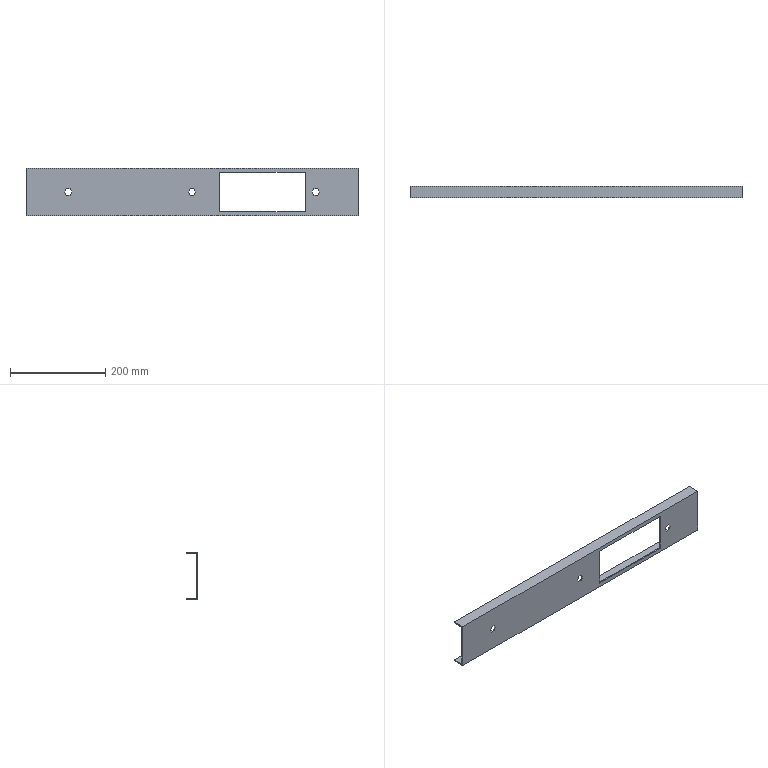Part | SolidWorks | features BaseBody 1 | 1 solid | 32 faces | box 698 x 25 x 100 mm | volume 215027 mm3 | plane 32
STEP:
#1=CARTESIAN_POINT('',(895.946,-3638.473,1001.471));
#2=VERTEX_POINT('',#1);
#3=CARTESIAN_POINT('',(895.946,-3638.473,1101.471));
#4=VERTEX_POINT('',#3);
#5=CARTESIAN_POINT('',(895.946,-3638.473,1081.471));
#6=DIRECTION('',(0.,0.,1.));
#7=VECTOR('',#6,1000.);
#8=LINE('',#5,#7);
#9=EDGE_CURVE('',#2,#4,#8,.T.);
#10=ORIENTED_EDGE('',*,*,#9,.T.);
#11=CARTESIAN_POINT('',(197.946,-3638.473,1101.471));
#12=VERTEX_POINT('',#11);
#13=CARTESIAN_POINT('',(895.946,-3638.473,1101.471));
#14=DIRECTION('',(-1.,0.,0.));
#15=VECTOR('',#14,1000.);
#16=LINE('',#13,#15);
#17=EDGE_CURVE('',#4,#12,#16,.T.);
#18=ORIENTED_EDGE('',*,*,#17,.T.);
#19=CARTESIAN_POINT('',(197.946,-3638.473,1001.471));
#20=VERTEX_POINT('',#19);
#21=CARTESIAN_POINT('',(197.946,-3638.473,1081.471));
#22=DIRECTION('',(0.,0.,-1.));
#23=VECTOR('',#22,1000.);
#24=LINE('',#21,#23);
#25=EDGE_CURVE('',#12,#20,#24,.T.);
#26=ORIENTED_EDGE('',*,*,#25,.T.);
#27=CARTESIAN_POINT('',(895.946,-3638.473,1001.471));
#28=DIRECTION('',(1.,0.,0.));
#29=VECTOR('',#28,1000.);
#30=LINE('',#27,#29);
#31=EDGE_CURVE('',#20,#2,#30,.T.);
#32=ORIENTED_EDGE('',*,*,#31,.T.);
#33=EDGE_LOOP('',(#10,#18,#26,#32));
#34=FACE_OUTER_BOUND('',#33,.T.);
#35=CARTESIAN_POINT('',(543.193,-3638.473,1044.971));
#36=VERTEX_POINT('',#35);
#37=CARTESIAN_POINT('',(539.44,-3638.473,1051.471));
#38=VERTEX_POINT('',#37);
#39=CARTESIAN_POINT('',(543.193,-3638.473,1044.971));
#40=DIRECTION('',(-0.5,0.,0.866));
#41=VECTOR('',#40,1000.);
#42=LINE('',#39,#41);
#43=EDGE_CURVE('',#36,#38,#42,.T.);
#44=ORIENTED_EDGE('',*,*,#43,.T.);
#45=CARTESIAN_POINT('',(543.193,-3638.473,1057.971));
#46=VERTEX_POINT('',#45);
#47=CARTESIAN_POINT('',(539.44,-3638.473,1051.471));
#48=DIRECTION('',(0.5,0.,0.866));
#49=VECTOR('',#48,1000.);
#50=LINE('',#47,#49);
#51=EDGE_CURVE('',#38,#46,#50,.T.);
#52=ORIENTED_EDGE('',*,*,#51,.T.);
#53=CARTESIAN_POINT('',(550.698,-3638.473,1057.971));
#54=VERTEX_POINT('',#53);
#55=CARTESIAN_POINT('',(895.946,-3638.473,1057.971));
#56=DIRECTION('',(1.,0.,0.));
#57=VECTOR('',#56,1000.);
#58=LINE('',#55,#57);
#59=EDGE_CURVE('',#46,#54,#58,.T.);
#60=ORIENTED_EDGE('',*,*,#59,.T.);
#61=CARTESIAN_POINT('',(554.451,-3638.473,1051.471));
#62=VERTEX_POINT('',#61);
#63=CARTESIAN_POINT('',(550.698,-3638.473,1057.971));
#64=DIRECTION('',(0.5,0.,-0.866));
#65=VECTOR('',#64,1000.);
#66=LINE('',#63,#65);
#67=EDGE_CURVE('',#54,#62,#66,.T.);
#68=ORIENTED_EDGE('',*,*,#67,.T.);
#69=CARTESIAN_POINT('',(550.698,-3638.473,1044.971));
#70=VERTEX_POINT('',#69);
#71=CARTESIAN_POINT('',(554.451,-3638.473,1051.471));
#72=DIRECTION('',(-0.5,0.,-0.866));
#73=VECTOR('',#72,1000.);
#74=LINE('',#71,#73);
#75=EDGE_CURVE('',#62,#70,#74,.T.);
#76=ORIENTED_EDGE('',*,*,#75,.T.);
#77=CARTESIAN_POINT('',(895.946,-3638.473,1044.971));
#78=DIRECTION('',(-1.,0.,0.));
#79=VECTOR('',#78,1000.);
#80=LINE('',#77,#79);
#81=EDGE_CURVE('',#70,#36,#80,.T.);
#82=ORIENTED_EDGE('',*,*,#81,.T.);
#83=EDGE_LOOP('',(#44,#52,#60,#68,#76,#82));
#84=FACE_BOUND('',#83,.T.);
#85=CARTESIAN_POINT('',(803.193,-3638.473,1044.971));
#86=VERTEX_POINT('',#85);
#87=CARTESIAN_POINT('',(799.44,-3638.473,1051.471));
#88=VERTEX_POINT('',#87);
#89=CARTESIAN_POINT('',(803.193,-3638.473,1044.971));
#90=DIRECTION('',(-0.5,0.,0.866));
#91=VECTOR('',#90,1000.);
#92=LINE('',#89,#91);
#93=EDGE_CURVE('',#86,#88,#92,.T.);
#94=ORIENTED_EDGE('',*,*,#93,.T.);
#95=CARTESIAN_POINT('',(803.193,-3638.473,1057.971));
#96=VERTEX_POINT('',#95);
#97=CARTESIAN_POINT('',(799.44,-3638.473,1051.471));
#98=DIRECTION('',(0.5,0.,0.866));
#99=VECTOR('',#98,1000.);
#100=LINE('',#97,#99);
#101=EDGE_CURVE('',#88,#96,#100,.T.);
#102=ORIENTED_EDGE('',*,*,#101,.T.);
#103=CARTESIAN_POINT('',(810.698,-3638.473,1057.971));
#104=VERTEX_POINT('',#103);
#105=CARTESIAN_POINT('',(895.946,-3638.473,1057.971));
#106=DIRECTION('',(1.,0.,0.));
#107=VECTOR('',#106,1000.);
#108=LINE('',#105,#107);
#109=EDGE_CURVE('',#96,#104,#108,.T.);
#110=ORIENTED_EDGE('',*,*,#109,.T.);
#111=CARTESIAN_POINT('',(814.451,-3638.473,1051.471));
#112=VERTEX_POINT('',#111);
#113=CARTESIAN_POINT('',(810.698,-3638.473,1057.971));
#114=DIRECTION('',(0.5,0.,-0.866));
#115=VECTOR('',#114,1000.);
#116=LINE('',#113,#115);
#117=EDGE_CURVE('',#104,#112,#116,.T.);
#118=ORIENTED_EDGE('',*,*,#117,.T.);
#119=CARTESIAN_POINT('',(810.698,-3638.473,1044.971));
#120=VERTEX_POINT('',#119);
#121=CARTESIAN_POINT('',(814.451,-3638.473,1051.471));
#122=DIRECTION('',(-0.5,0.,-0.866));
#123=VECTOR('',#122,1000.);
#124=LINE('',#121,#123);
#125=EDGE_CURVE('',#112,#120,#124,.T.);
#126=ORIENTED_EDGE('',*,*,#125,.T.);
#127=CARTESIAN_POINT('',(895.946,-3638.473,1044.971));
#128=DIRECTION('',(-1.,0.,0.));
#129=VECTOR('',#128,1000.);
#130=LINE('',#127,#129);
#131=EDGE_CURVE('',#120,#86,#130,.T.);
#132=ORIENTED_EDGE('',*,*,#131,.T.);
#133=EDGE_LOOP('',(#94,#102,#110,#118,#126,#132));
#134=FACE_BOUND('',#133,.T.);
#135=CARTESIAN_POINT('',(283.193,-3638.473,1044.971));
#136=VERTEX_POINT('',#135);
#137=CARTESIAN_POINT('',(279.44,-3638.473,1051.471));
#138=VERTEX_POINT('',#137);
#139=CARTESIAN_POINT('',(283.193,-3638.473,1044.971));
#140=DIRECTION('',(-0.5,0.,0.866));
#141=VECTOR('',#140,1000.);
#142=LINE('',#139,#141);
#143=EDGE_CURVE('',#136,#138,#142,.T.);
#144=ORIENTED_EDGE('',*,*,#143,.T.);
#145=CARTESIAN_POINT('',(283.193,-3638.473,1057.971));
#146=VERTEX_POINT('',#145);
#147=CARTESIAN_POINT('',(279.44,-3638.473,1051.471));
#148=DIRECTION('',(0.5,0.,0.866));
#149=VECTOR('',#148,1000.);
#150=LINE('',#147,#149);
#151=EDGE_CURVE('',#138,#146,#150,.T.);
#152=ORIENTED_EDGE('',*,*,#151,.T.);
#153=CARTESIAN_POINT('',(290.698,-3638.473,1057.971));
#154=VERTEX_POINT('',#153);
#155=CARTESIAN_POINT('',(895.946,-3638.473,1057.971));
#156=DIRECTION('',(1.,0.,0.));
#157=VECTOR('',#156,1000.);
#158=LINE('',#155,#157);
#159=EDGE_CURVE('',#146,#154,#158,.T.);
#160=ORIENTED_EDGE('',*,*,#159,.T.);
#161=CARTESIAN_POINT('',(294.451,-3638.473,1051.471));
#162=VERTEX_POINT('',#161);
#163=CARTESIAN_POINT('',(290.698,-3638.473,1057.971));
#164=DIRECTION('',(0.5,0.,-0.866));
#165=VECTOR('',#164,1000.);
#166=LINE('',#163,#165);
#167=EDGE_CURVE('',#154,#162,#166,.T.);
#168=ORIENTED_EDGE('',*,*,#167,.T.);
#169=CARTESIAN_POINT('',(290.698,-3638.473,1044.971));
#170=VERTEX_POINT('',#169);
#171=CARTESIAN_POINT('',(294.451,-3638.473,1051.471));
#172=DIRECTION('',(-0.5,0.,-0.866));
#173=VECTOR('',#172,1000.);
#174=LINE('',#171,#173);
#175=EDGE_CURVE('',#162,#170,#174,.T.);
#176=ORIENTED_EDGE('',*,*,#175,.T.);
#177=CARTESIAN_POINT('',(895.946,-3638.473,1044.971));
#178=DIRECTION('',(-1.,0.,0.));
#179=VECTOR('',#178,1000.);
#180=LINE('',#177,#179);
#181=EDGE_CURVE('',#170,#136,#180,.T.);
#182=ORIENTED_EDGE('',*,*,#181,.T.);
#183=EDGE_LOOP('',(#144,#152,#160,#168,#176,#182));
#184=FACE_BOUND('',#183,.T.);
#185=CARTESIAN_POINT('',(784.946,-3638.473,1092.471));
#186=VERTEX_POINT('',#185);
#187=CARTESIAN_POINT('',(784.946,-3638.473,1010.471));
#188=VERTEX_POINT('',#187);
#189=CARTESIAN_POINT('',(784.946,-3638.473,1081.471));
#190=DIRECTION('',(0.,0.,-1.));
#191=VECTOR('',#190,1000.);
#192=LINE('',#189,#191);
#193=EDGE_CURVE('',#186,#188,#192,.T.);
#194=ORIENTED_EDGE('',*,*,#193,.T.);
#195=CARTESIAN_POINT('',(604.946,-3638.473,1010.471));
#196=VERTEX_POINT('',#195);
#197=CARTESIAN_POINT('',(895.946,-3638.473,1010.471));
#198=DIRECTION('',(-1.,0.,0.));
#199=VECTOR('',#198,1000.);
#200=LINE('',#197,#199);
#201=EDGE_CURVE('',#188,#196,#200,.T.);
#202=ORIENTED_EDGE('',*,*,#201,.T.);
#203=CARTESIAN_POINT('',(604.946,-3638.473,1092.471));
#204=VERTEX_POINT('',#203);
#205=CARTESIAN_POINT('',(604.946,-3638.473,1081.471));
#206=DIRECTION('',(0.,0.,1.));
#207=VECTOR('',#206,1000.);
#208=LINE('',#205,#207);
#209=EDGE_CURVE('',#196,#204,#208,.T.);
#210=ORIENTED_EDGE('',*,*,#209,.T.);
#211=CARTESIAN_POINT('',(895.946,-3638.473,1092.471));
#212=DIRECTION('',(1.,0.,0.));
#213=VECTOR('',#212,1000.);
#214=LINE('',#211,#213);
#215=EDGE_CURVE('',#204,#186,#214,.T.);
#216=ORIENTED_EDGE('',*,*,#215,.T.);
#217=EDGE_LOOP('',(#194,#202,#210,#216));
#218=FACE_BOUND('',#217,.T.);
#219=CARTESIAN_POINT('',(895.946,-3638.473,1081.471));
#220=DIRECTION('',(0.,-1.,0.));
#221=DIRECTION('',(0.,0.,-1.));
#222=AXIS2_PLACEMENT_3D('',#219,#220,#221);
#223=PLANE('',#222);
#224=ADVANCED_FACE('',(#34,#84,#134,#184,#218),#223,.T.);
#225=CARTESIAN_POINT('',(895.946,-3613.473,1101.471));
#226=VERTEX_POINT('',#225);
#227=CARTESIAN_POINT('',(895.946,-3613.473,1101.471));
#228=DIRECTION('',(0.,1.,0.));
#229=VECTOR('',#228,1000.);
#230=LINE('',#227,#229);
#231=EDGE_CURVE('',#4,#226,#230,.T.);
#232=ORIENTED_EDGE('',*,*,#231,.T.);
#233=CARTESIAN_POINT('',(197.946,-3613.473,1101.471));
#234=VERTEX_POINT('',#233);
#235=CARTESIAN_POINT('',(895.946,-3613.473,1101.471));
#236=DIRECTION('',(-1.,0.,0.));
#237=VECTOR('',#236,1000.);
#238=LINE('',#235,#237);
#239=EDGE_CURVE('',#226,#234,#238,.T.);
#240=ORIENTED_EDGE('',*,*,#239,.T.);
#241=CARTESIAN_POINT('',(197.946,-3613.473,1101.471));
#242=DIRECTION('',(0.,-1.,0.));
#243=VECTOR('',#242,1000.);
#244=LINE('',#241,#243);
#245=EDGE_CURVE('',#234,#12,#244,.T.);
#246=ORIENTED_EDGE('',*,*,#245,.T.);
#247=ORIENTED_EDGE('',*,*,#17,.F.);
#248=EDGE_LOOP('',(#232,#240,#246,#247));
#249=FACE_OUTER_BOUND('',#248,.T.);
#250=CARTESIAN_POINT('',(895.946,-3613.473,1101.471));
#251=DIRECTION('',(0.,0.,1.));
#252=DIRECTION('',(1.,0.,0.));
#253=AXIS2_PLACEMENT_3D('',#250,#251,#252);
#254=PLANE('',#253);
#255=ADVANCED_FACE('',(#249),#254,.T.);
#256=CARTESIAN_POINT('',(895.946,-3613.473,1001.471));
#257=VERTEX_POINT('',#256);
#258=CARTESIAN_POINT('',(895.946,-3631.467,1001.471));
#259=DIRECTION('',(0.,1.,0.));
#260=VECTOR('',#259,1000.);
#261=LINE('',#258,#260);
#262=EDGE_CURVE('',#2,#257,#261,.T.);
#263=ORIENTED_EDGE('',*,*,#262,.T.);
#264=CARTESIAN_POINT('',(895.946,-3613.473,1003.971));
#265=VERTEX_POINT('',#264);
#266=CARTESIAN_POINT('',(895.946,-3613.473,1051.471));
#267=DIRECTION('',(0.,0.,1.));
#268=VECTOR('',#267,1000.);
#269=LINE('',#266,#268);
#270=EDGE_CURVE('',#257,#265,#269,.T.);
#271=ORIENTED_EDGE('',*,*,#270,.T.);
#272=CARTESIAN_POINT('',(895.946,-3635.973,1003.971));
#273=VERTEX_POINT('',#272);
#274=CARTESIAN_POINT('',(895.946,-3631.467,1003.971));
#275=DIRECTION('',(0.,-1.,0.));
#276=VECTOR('',#275,1000.);
#277=LINE('',#274,#276);
#278=EDGE_CURVE('',#265,#273,#277,.T.);
#279=ORIENTED_EDGE('',*,*,#278,.T.);
#280=CARTESIAN_POINT('',(895.946,-3635.973,1098.971));
#281=VERTEX_POINT('',#280);
#282=CARTESIAN_POINT('',(895.946,-3635.973,1051.471));
#283=DIRECTION('',(0.,0.,1.));
#284=VECTOR('',#283,1000.);
#285=LINE('',#282,#284);
#286=EDGE_CURVE('',#273,#281,#285,.T.);
#287=ORIENTED_EDGE('',*,*,#286,.T.);
#288=CARTESIAN_POINT('',(895.946,-3613.473,1098.971));
#289=VERTEX_POINT('',#288);
#290=CARTESIAN_POINT('',(895.946,-3631.467,1098.971));
#291=DIRECTION('',(0.,1.,0.));
#292=VECTOR('',#291,1000.);
#293=LINE('',#290,#292);
#294=EDGE_CURVE('',#281,#289,#293,.T.);
#295=ORIENTED_EDGE('',*,*,#294,.T.);
#296=CARTESIAN_POINT('',(895.946,-3613.473,1051.471));
#297=DIRECTION('',(0.,0.,1.));
#298=VECTOR('',#297,1000.);
#299=LINE('',#296,#298);
#300=EDGE_CURVE('',#289,#226,#299,.T.);
#301=ORIENTED_EDGE('',*,*,#300,.T.);
#302=ORIENTED_EDGE('',*,*,#231,.F.);
#303=ORIENTED_EDGE('',*,*,#9,.F.);
#304=EDGE_LOOP('',(#263,#271,#279,#287,#295,#301,#302,#303));
#305=FACE_OUTER_BOUND('',#304,.T.);
#306=CARTESIAN_POINT('',(895.946,-3631.467,1051.471));
#307=DIRECTION('',(1.,0.,0.));
#308=DIRECTION('',(0.,0.,-1.));
#309=AXIS2_PLACEMENT_3D('',#306,#307,#308);
#310=PLANE('',#309);
#311=ADVANCED_FACE('',(#305),#310,.T.);
#312=ORIENTED_EDGE('',*,*,#262,.F.);
#313=ORIENTED_EDGE('',*,*,#31,.F.);
#314=CARTESIAN_POINT('',(197.946,-3613.473,1001.471));
#315=VERTEX_POINT('',#314);
#316=CARTESIAN_POINT('',(197.946,-3638.473,1001.471));
#317=DIRECTION('',(0.,1.,0.));
#318=VECTOR('',#317,1000.);
#319=LINE('',#316,#318);
#320=EDGE_CURVE('',#20,#315,#319,.T.);
#321=ORIENTED_EDGE('',*,*,#320,.T.);
#322=CARTESIAN_POINT('',(895.946,-3613.473,1001.471));
#323=DIRECTION('',(1.,0.,0.));
#324=VECTOR('',#323,1000.);
#325=LINE('',#322,#324);
#326=EDGE_CURVE('',#315,#257,#325,.T.);
#327=ORIENTED_EDGE('',*,*,#326,.T.);
#328=EDGE_LOOP('',(#312,#313,#321,#327));
#329=FACE_OUTER_BOUND('',#328,.T.);
#330=CARTESIAN_POINT('',(895.946,-3638.473,1001.471));
#331=DIRECTION('',(0.,0.,-1.));
#332=DIRECTION('',(-1.,0.,0.));
#333=AXIS2_PLACEMENT_3D('',#330,#331,#332);
#334=PLANE('',#333);
#335=ADVANCED_FACE('',(#329),#334,.T.);
#336=CARTESIAN_POINT('',(197.946,-3613.473,1003.971));
#337=VERTEX_POINT('',#336);
#338=CARTESIAN_POINT('',(197.946,-3635.973,1003.971));
#339=VERTEX_POINT('',#338);
#340=CARTESIAN_POINT('',(197.946,-3631.467,1003.971));
#341=DIRECTION('',(0.,-1.,0.));
#342=VECTOR('',#341,1000.);
#343=LINE('',#340,#342);
#344=EDGE_CURVE('',#337,#339,#343,.T.);
#345=ORIENTED_EDGE('',*,*,#344,.F.);
#346=CARTESIAN_POINT('',(197.946,-3613.473,1051.471));
#347=DIRECTION('',(0.,0.,1.));
#348=VECTOR('',#347,1000.);
#349=LINE('',#346,#348);
#350=EDGE_CURVE('',#315,#337,#349,.T.);
#351=ORIENTED_EDGE('',*,*,#350,.F.);
#352=ORIENTED_EDGE('',*,*,#320,.F.);
#353=ORIENTED_EDGE('',*,*,#25,.F.);
#354=ORIENTED_EDGE('',*,*,#245,.F.);
#355=CARTESIAN_POINT('',(197.946,-3613.473,1098.971));
#356=VERTEX_POINT('',#355);
#357=CARTESIAN_POINT('',(197.946,-3613.473,1051.471));
#358=DIRECTION('',(0.,0.,1.));
#359=VECTOR('',#358,1000.);
#360=LINE('',#357,#359);
#361=EDGE_CURVE('',#356,#234,#360,.T.);
#362=ORIENTED_EDGE('',*,*,#361,.F.);
#363=CARTESIAN_POINT('',(197.946,-3635.973,1098.971));
#364=VERTEX_POINT('',#363);
#365=CARTESIAN_POINT('',(197.946,-3631.467,1098.971));
#366=DIRECTION('',(0.,1.,0.));
#367=VECTOR('',#366,1000.);
#368=LINE('',#365,#367);
#369=EDGE_CURVE('',#364,#356,#368,.T.);
#370=ORIENTED_EDGE('',*,*,#369,.F.);
#371=CARTESIAN_POINT('',(197.946,-3635.973,1051.471));
#372=DIRECTION('',(0.,0.,1.));
#373=VECTOR('',#372,1000.);
#374=LINE('',#371,#373);
#375=EDGE_CURVE('',#339,#364,#374,.T.);
#376=ORIENTED_EDGE('',*,*,#375,.F.);
#377=EDGE_LOOP('',(#345,#351,#352,#353,#354,#362,#370,#376));
#378=FACE_OUTER_BOUND('',#377,.T.);
#379=CARTESIAN_POINT('',(197.946,-3631.467,1051.471));
#380=DIRECTION('',(1.,0.,0.));
#381=DIRECTION('',(0.,0.,-1.));
#382=AXIS2_PLACEMENT_3D('',#379,#380,#381);
#383=PLANE('',#382);
#384=ADVANCED_FACE('',(#378),#383,.F.);
#385=CARTESIAN_POINT('',(543.193,-3635.973,1057.971));
#386=VERTEX_POINT('',#385);
#387=CARTESIAN_POINT('',(543.193,-3609.088,1057.971));
#388=DIRECTION('',(0.,1.,0.));
#389=VECTOR('',#388,1000.);
#390=LINE('',#387,#389);
#391=EDGE_CURVE('',#46,#386,#390,.T.);
#392=ORIENTED_EDGE('',*,*,#391,.F.);
#393=ORIENTED_EDGE('',*,*,#51,.F.);
#394=CARTESIAN_POINT('',(539.44,-3635.973,1051.471));
#395=VERTEX_POINT('',#394);
#396=CARTESIAN_POINT('',(539.44,-3609.088,1051.471));
#397=DIRECTION('',(0.,-1.,0.));
#398=VECTOR('',#397,1000.);
#399=LINE('',#396,#398);
#400=EDGE_CURVE('',#395,#38,#399,.T.);
#401=ORIENTED_EDGE('',*,*,#400,.F.);
#402=CARTESIAN_POINT('',(539.44,-3635.973,1051.471));
#403=DIRECTION('',(-0.5,0.,-0.866));
#404=VECTOR('',#403,1000.);
#405=LINE('',#402,#404);
#406=EDGE_CURVE('',#386,#395,#405,.T.);
#407=ORIENTED_EDGE('',*,*,#406,.F.);
#408=EDGE_LOOP('',(#392,#393,#401,#407));
#409=FACE_OUTER_BOUND('',#408,.T.);
#410=CARTESIAN_POINT('',(539.44,-3609.088,1051.471));
#411=DIRECTION('',(-0.866,0.,0.5));
#412=DIRECTION('',(0.5,0.,0.866));
#413=AXIS2_PLACEMENT_3D('',#410,#411,#412);
#414=PLANE('',#413);
#415=ADVANCED_FACE('',(#409),#414,.F.);
#416=ORIENTED_EDGE('',*,*,#400,.T.);
#417=ORIENTED_EDGE('',*,*,#43,.F.);
#418=CARTESIAN_POINT('',(543.193,-3635.973,1044.971));
#419=VERTEX_POINT('',#418);
#420=CARTESIAN_POINT('',(543.193,-3609.088,1044.971));
#421=DIRECTION('',(0.,-1.,0.));
#422=VECTOR('',#421,1000.);
#423=LINE('',#420,#422);
#424=EDGE_CURVE('',#419,#36,#423,.T.);
#425=ORIENTED_EDGE('',*,*,#424,.F.);
#426=CARTESIAN_POINT('',(543.193,-3635.973,1044.971));
#427=DIRECTION('',(0.5,0.,-0.866));
#428=VECTOR('',#427,1000.);
#429=LINE('',#426,#428);
#430=EDGE_CURVE('',#395,#419,#429,.T.);
#431=ORIENTED_EDGE('',*,*,#430,.F.);
#432=EDGE_LOOP('',(#416,#417,#425,#431));
#433=FACE_OUTER_BOUND('',#432,.T.);
#434=CARTESIAN_POINT('',(543.193,-3609.088,1044.971));
#435=DIRECTION('',(-0.866,0.,-0.5));
#436=DIRECTION('',(-0.5,0.,0.866));
#437=AXIS2_PLACEMENT_3D('',#434,#435,#436);
#438=PLANE('',#437);
#439=ADVANCED_FACE('',(#433),#438,.F.);
#440=ORIENTED_EDGE('',*,*,#424,.T.);
#441=ORIENTED_EDGE('',*,*,#81,.F.);
#442=CARTESIAN_POINT('',(550.698,-3635.973,1044.971));
#443=VERTEX_POINT('',#442);
#444=CARTESIAN_POINT('',(550.698,-3609.088,1044.971));
#445=DIRECTION('',(0.,-1.,0.));
#446=VECTOR('',#445,1000.);
#447=LINE('',#444,#446);
#448=EDGE_CURVE('',#443,#70,#447,.T.);
#449=ORIENTED_EDGE('',*,*,#448,.F.);
#450=CARTESIAN_POINT('',(550.698,-3635.973,1044.971));
#451=DIRECTION('',(1.,0.,0.));
#452=VECTOR('',#451,1000.);
#453=LINE('',#450,#452);
#454=EDGE_CURVE('',#419,#443,#453,.T.);
#455=ORIENTED_EDGE('',*,*,#454,.F.);
#456=EDGE_LOOP('',(#440,#441,#449,#455));
#457=FACE_OUTER_BOUND('',#456,.T.);
#458=CARTESIAN_POINT('',(550.698,-3609.088,1044.971));
#459=DIRECTION('',(0.,0.,-1.));
#460=DIRECTION('',(-1.,0.,0.));
#461=AXIS2_PLACEMENT_3D('',#458,#459,#460);
#462=PLANE('',#461);
#463=ADVANCED_FACE('',(#457),#462,.F.);
#464=ORIENTED_EDGE('',*,*,#448,.T.);
#465=ORIENTED_EDGE('',*,*,#75,.F.);
#466=CARTESIAN_POINT('',(554.451,-3635.973,1051.471));
#467=VERTEX_POINT('',#466);
#468=CARTESIAN_POINT('',(554.451,-3609.088,1051.471));
#469=DIRECTION('',(0.,-1.,0.));
#470=VECTOR('',#469,1000.);
#471=LINE('',#468,#470);
#472=EDGE_CURVE('',#467,#62,#471,.T.);
#473=ORIENTED_EDGE('',*,*,#472,.F.);
#474=CARTESIAN_POINT('',(554.451,-3635.973,1051.471));
#475=DIRECTION('',(0.5,0.,0.866));
#476=VECTOR('',#475,1000.);
#477=LINE('',#474,#476);
#478=EDGE_CURVE('',#443,#467,#477,.T.);
#479=ORIENTED_EDGE('',*,*,#478,.F.);
#480=EDGE_LOOP('',(#464,#465,#473,#479));
#481=FACE_OUTER_BOUND('',#480,.T.);
#482=CARTESIAN_POINT('',(554.451,-3609.088,1051.471));
#483=DIRECTION('',(0.866,0.,-0.5));
#484=DIRECTION('',(-0.5,0.,-0.866));
#485=AXIS2_PLACEMENT_3D('',#482,#483,#484);
#486=PLANE('',#485);
#487=ADVANCED_FACE('',(#481),#486,.F.);
#488=ORIENTED_EDGE('',*,*,#472,.T.);
#489=ORIENTED_EDGE('',*,*,#67,.F.);
#490=CARTESIAN_POINT('',(550.698,-3635.973,1057.971));
#491=VERTEX_POINT('',#490);
#492=CARTESIAN_POINT('',(550.698,-3609.088,1057.971));
#493=DIRECTION('',(0.,-1.,0.));
#494=VECTOR('',#493,1000.);
#495=LINE('',#492,#494);
#496=EDGE_CURVE('',#491,#54,#495,.T.);
#497=ORIENTED_EDGE('',*,*,#496,.F.);
#498=CARTESIAN_POINT('',(550.698,-3635.973,1057.971));
#499=DIRECTION('',(-0.5,0.,0.866));
#500=VECTOR('',#499,1000.);
#501=LINE('',#498,#500);
#502=EDGE_CURVE('',#467,#491,#501,.T.);
#503=ORIENTED_EDGE('',*,*,#502,.F.);
#504=EDGE_LOOP('',(#488,#489,#497,#503));
#505=FACE_OUTER_BOUND('',#504,.T.);
#506=CARTESIAN_POINT('',(550.698,-3609.088,1057.971));
#507=DIRECTION('',(0.866,0.,0.5));
#508=DIRECTION('',(0.5,0.,-0.866));
#509=AXIS2_PLACEMENT_3D('',#506,#507,#508);
#510=PLANE('',#509);
#511=ADVANCED_FACE('',(#505),#510,.F.);
#512=ORIENTED_EDGE('',*,*,#496,.T.);
#513=ORIENTED_EDGE('',*,*,#59,.F.);
#514=ORIENTED_EDGE('',*,*,#391,.T.);
#515=CARTESIAN_POINT('',(543.193,-3635.973,1057.971));
#516=DIRECTION('',(-1.,0.,0.));
#517=VECTOR('',#516,1000.);
#518=LINE('',#515,#517);
#519=EDGE_CURVE('',#491,#386,#518,.T.);
#520=ORIENTED_EDGE('',*,*,#519,.F.);
#521=EDGE_LOOP('',(#512,#513,#514,#520));
#522=FACE_OUTER_BOUND('',#521,.T.);
#523=CARTESIAN_POINT('',(543.193,-3609.088,1057.971));
#524=DIRECTION('',(0.,0.,1.));
#525=DIRECTION('',(1.,0.,0.));
#526=AXIS2_PLACEMENT_3D('',#523,#524,#525);
#527=PLANE('',#526);
#528=ADVANCED_FACE('',(#522),#527,.F.);
#529=CARTESIAN_POINT('',(803.193,-3635.973,1057.971));
#530=VERTEX_POINT('',#529);
#531=CARTESIAN_POINT('',(803.193,-3609.088,1057.971));
#532=DIRECTION('',(0.,1.,0.));
#533=VECTOR('',#532,1000.);
#534=LINE('',#531,#533);
#535=EDGE_CURVE('',#96,#530,#534,.T.);
#536=ORIENTED_EDGE('',*,*,#535,.F.);
#537=ORIENTED_EDGE('',*,*,#101,.F.);
#538=CARTESIAN_POINT('',(799.44,-3635.973,1051.471));
#539=VERTEX_POINT('',#538);
#540=CARTESIAN_POINT('',(799.44,-3609.088,1051.471));
#541=DIRECTION('',(0.,-1.,0.));
#542=VECTOR('',#541,1000.);
#543=LINE('',#540,#542);
#544=EDGE_CURVE('',#539,#88,#543,.T.);
#545=ORIENTED_EDGE('',*,*,#544,.F.);
#546=CARTESIAN_POINT('',(799.44,-3635.973,1051.471));
#547=DIRECTION('',(-0.5,0.,-0.866));
#548=VECTOR('',#547,1000.);
#549=LINE('',#546,#548);
#550=EDGE_CURVE('',#530,#539,#549,.T.);
#551=ORIENTED_EDGE('',*,*,#550,.F.);
#552=EDGE_LOOP('',(#536,#537,#545,#551));
#553=FACE_OUTER_BOUND('',#552,.T.);
#554=CARTESIAN_POINT('',(799.44,-3609.088,1051.471));
#555=DIRECTION('',(-0.866,0.,0.5));
#556=DIRECTION('',(0.5,0.,0.866));
#557=AXIS2_PLACEMENT_3D('',#554,#555,#556);
#558=PLANE('',#557);
#559=ADVANCED_FACE('',(#553),#558,.F.);
#560=ORIENTED_EDGE('',*,*,#544,.T.);
#561=ORIENTED_EDGE('',*,*,#93,.F.);
#562=CARTESIAN_POINT('',(803.193,-3635.973,1044.971));
#563=VERTEX_POINT('',#562);
#564=CARTESIAN_POINT('',(803.193,-3609.088,1044.971));
#565=DIRECTION('',(0.,-1.,0.));
#566=VECTOR('',#565,1000.);
#567=LINE('',#564,#566);
#568=EDGE_CURVE('',#563,#86,#567,.T.);
#569=ORIENTED_EDGE('',*,*,#568,.F.);
#570=CARTESIAN_POINT('',(803.193,-3635.973,1044.971));
#571=DIRECTION('',(0.5,0.,-0.866));
#572=VECTOR('',#571,1000.);
#573=LINE('',#570,#572);
#574=EDGE_CURVE('',#539,#563,#573,.T.);
#575=ORIENTED_EDGE('',*,*,#574,.F.);
#576=EDGE_LOOP('',(#560,#561,#569,#575));
#577=FACE_OUTER_BOUND('',#576,.T.);
#578=CARTESIAN_POINT('',(803.193,-3609.088,1044.971));
#579=DIRECTION('',(-0.866,0.,-0.5));
#580=DIRECTION('',(-0.5,0.,0.866));
#581=AXIS2_PLACEMENT_3D('',#578,#579,#580);
#582=PLANE('',#581);
#583=ADVANCED_FACE('',(#577),#582,.F.);
#584=ORIENTED_EDGE('',*,*,#568,.T.);
#585=ORIENTED_EDGE('',*,*,#131,.F.);
#586=CARTESIAN_POINT('',(810.698,-3635.973,1044.971));
#587=VERTEX_POINT('',#586);
#588=CARTESIAN_POINT('',(810.698,-3609.088,1044.971));
#589=DIRECTION('',(0.,-1.,0.));
#590=VECTOR('',#589,1000.);
#591=LINE('',#588,#590);
#592=EDGE_CURVE('',#587,#120,#591,.T.);
#593=ORIENTED_EDGE('',*,*,#592,.F.);
#594=CARTESIAN_POINT('',(810.698,-3635.973,1044.971));
#595=DIRECTION('',(1.,0.,0.));
#596=VECTOR('',#595,1000.);
#597=LINE('',#594,#596);
#598=EDGE_CURVE('',#563,#587,#597,.T.);
#599=ORIENTED_EDGE('',*,*,#598,.F.);
#600=EDGE_LOOP('',(#584,#585,#593,#599));
#601=FACE_OUTER_BOUND('',#600,.T.);
#602=CARTESIAN_POINT('',(810.698,-3609.088,1044.971));
#603=DIRECTION('',(0.,0.,-1.));
#604=DIRECTION('',(-1.,0.,0.));
#605=AXIS2_PLACEMENT_3D('',#602,#603,#604);
#606=PLANE('',#605);
#607=ADVANCED_FACE('',(#601),#606,.F.);
#608=ORIENTED_EDGE('',*,*,#592,.T.);
#609=ORIENTED_EDGE('',*,*,#125,.F.);
#610=CARTESIAN_POINT('',(814.451,-3635.973,1051.471));
#611=VERTEX_POINT('',#610);
#612=CARTESIAN_POINT('',(814.451,-3609.088,1051.471));
#613=DIRECTION('',(0.,-1.,0.));
#614=VECTOR('',#613,1000.);
#615=LINE('',#612,#614);
#616=EDGE_CURVE('',#611,#112,#615,.T.);
#617=ORIENTED_EDGE('',*,*,#616,.F.);
#618=CARTESIAN_POINT('',(814.451,-3635.973,1051.471));
#619=DIRECTION('',(0.5,0.,0.866));
#620=VECTOR('',#619,1000.);
#621=LINE('',#618,#620);
#622=EDGE_CURVE('',#587,#611,#621,.T.);
#623=ORIENTED_EDGE('',*,*,#622,.F.);
#624=EDGE_LOOP('',(#608,#609,#617,#623));
#625=FACE_OUTER_BOUND('',#624,.T.);
#626=CARTESIAN_POINT('',(814.451,-3609.088,1051.471));
#627=DIRECTION('',(0.866,0.,-0.5));
#628=DIRECTION('',(-0.5,0.,-0.866));
#629=AXIS2_PLACEMENT_3D('',#626,#627,#628);
#630=PLANE('',#629);
#631=ADVANCED_FACE('',(#625),#630,.F.);
#632=ORIENTED_EDGE('',*,*,#616,.T.);
#633=ORIENTED_EDGE('',*,*,#117,.F.);
#634=CARTESIAN_POINT('',(810.698,-3635.973,1057.971));
#635=VERTEX_POINT('',#634);
#636=CARTESIAN_POINT('',(810.698,-3609.088,1057.971));
#637=DIRECTION('',(0.,-1.,0.));
#638=VECTOR('',#637,1000.);
#639=LINE('',#636,#638);
#640=EDGE_CURVE('',#635,#104,#639,.T.);
#641=ORIENTED_EDGE('',*,*,#640,.F.);
#642=CARTESIAN_POINT('',(810.698,-3635.973,1057.971));
#643=DIRECTION('',(-0.5,0.,0.866));
#644=VECTOR('',#643,1000.);
#645=LINE('',#642,#644);
#646=EDGE_CURVE('',#611,#635,#645,.T.);
#647=ORIENTED_EDGE('',*,*,#646,.F.);
#648=EDGE_LOOP('',(#632,#633,#641,#647));
#649=FACE_OUTER_BOUND('',#648,.T.);
#650=CARTESIAN_POINT('',(810.698,-3609.088,1057.971));
#651=DIRECTION('',(0.866,0.,0.5));
#652=DIRECTION('',(0.5,0.,-0.866));
#653=AXIS2_PLACEMENT_3D('',#650,#651,#652);
#654=PLANE('',#653);
#655=ADVANCED_FACE('',(#649),#654,.F.);
#656=ORIENTED_EDGE('',*,*,#640,.T.);
#657=ORIENTED_EDGE('',*,*,#109,.F.);
#658=ORIENTED_EDGE('',*,*,#535,.T.);
#659=CARTESIAN_POINT('',(803.193,-3635.973,1057.971));
#660=DIRECTION('',(-1.,0.,0.));
#661=VECTOR('',#660,1000.);
#662=LINE('',#659,#661);
#663=EDGE_CURVE('',#635,#530,#662,.T.);
#664=ORIENTED_EDGE('',*,*,#663,.F.);
#665=EDGE_LOOP('',(#656,#657,#658,#664));
#666=FACE_OUTER_BOUND('',#665,.T.);
#667=CARTESIAN_POINT('',(803.193,-3609.088,1057.971));
#668=DIRECTION('',(0.,0.,1.));
#669=DIRECTION('',(1.,0.,0.));
#670=AXIS2_PLACEMENT_3D('',#667,#668,#669);
#671=PLANE('',#670);
#672=ADVANCED_FACE('',(#666),#671,.F.);
#673=CARTESIAN_POINT('',(283.193,-3635.973,1057.971));
#674=VERTEX_POINT('',#673);
#675=CARTESIAN_POINT('',(283.193,-3609.088,1057.971));
#676=DIRECTION('',(0.,1.,0.));
#677=VECTOR('',#676,1000.);
#678=LINE('',#675,#677);
#679=EDGE_CURVE('',#146,#674,#678,.T.);
#680=ORIENTED_EDGE('',*,*,#679,.F.);
#681=ORIENTED_EDGE('',*,*,#151,.F.);
#682=CARTESIAN_POINT('',(279.44,-3635.973,1051.471));
#683=VERTEX_POINT('',#682);
#684=CARTESIAN_POINT('',(279.44,-3609.088,1051.471));
#685=DIRECTION('',(0.,-1.,0.));
#686=VECTOR('',#685,1000.);
#687=LINE('',#684,#686);
#688=EDGE_CURVE('',#683,#138,#687,.T.);
#689=ORIENTED_EDGE('',*,*,#688,.F.);
#690=CARTESIAN_POINT('',(279.44,-3635.973,1051.471));
#691=DIRECTION('',(-0.5,0.,-0.866));
#692=VECTOR('',#691,1000.);
#693=LINE('',#690,#692);
#694=EDGE_CURVE('',#674,#683,#693,.T.);
#695=ORIENTED_EDGE('',*,*,#694,.F.);
#696=EDGE_LOOP('',(#680,#681,#689,#695));
#697=FACE_OUTER_BOUND('',#696,.T.);
#698=CARTESIAN_POINT('',(279.44,-3609.088,1051.471));
#699=DIRECTION('',(-0.866,0.,0.5));
#700=DIRECTION('',(0.5,0.,0.866));
#701=AXIS2_PLACEMENT_3D('',#698,#699,#700);
#702=PLANE('',#701);
#703=ADVANCED_FACE('',(#697),#702,.F.);
#704=ORIENTED_EDGE('',*,*,#688,.T.);
#705=ORIENTED_EDGE('',*,*,#143,.F.);
#706=CARTESIAN_POINT('',(283.193,-3635.973,1044.971));
#707=VERTEX_POINT('',#706);
#708=CARTESIAN_POINT('',(283.193,-3609.088,1044.971));
#709=DIRECTION('',(0.,-1.,0.));
#710=VECTOR('',#709,1000.);
#711=LINE('',#708,#710);
#712=EDGE_CURVE('',#707,#136,#711,.T.);
#713=ORIENTED_EDGE('',*,*,#712,.F.);
#714=CARTESIAN_POINT('',(283.193,-3635.973,1044.971));
#715=DIRECTION('',(0.5,0.,-0.866));
#716=VECTOR('',#715,1000.);
#717=LINE('',#714,#716);
#718=EDGE_CURVE('',#683,#707,#717,.T.);
#719=ORIENTED_EDGE('',*,*,#718,.F.);
#720=EDGE_LOOP('',(#704,#705,#713,#719));
#721=FACE_OUTER_BOUND('',#720,.T.);
#722=CARTESIAN_POINT('',(283.193,-3609.088,1044.971));
#723=DIRECTION('',(-0.866,0.,-0.5));
#724=DIRECTION('',(-0.5,0.,0.866));
#725=AXIS2_PLACEMENT_3D('',#722,#723,#724);
#726=PLANE('',#725);
#727=ADVANCED_FACE('',(#721),#726,.F.);
#728=ORIENTED_EDGE('',*,*,#712,.T.);
#729=ORIENTED_EDGE('',*,*,#181,.F.);
#730=CARTESIAN_POINT('',(290.698,-3635.973,1044.971));
#731=VERTEX_POINT('',#730);
#732=CARTESIAN_POINT('',(290.698,-3609.088,1044.971));
#733=DIRECTION('',(0.,-1.,0.));
#734=VECTOR('',#733,1000.);
#735=LINE('',#732,#734);
#736=EDGE_CURVE('',#731,#170,#735,.T.);
#737=ORIENTED_EDGE('',*,*,#736,.F.);
#738=CARTESIAN_POINT('',(290.698,-3635.973,1044.971));
#739=DIRECTION('',(1.,0.,0.));
#740=VECTOR('',#739,1000.);
#741=LINE('',#738,#740);
#742=EDGE_CURVE('',#707,#731,#741,.T.);
#743=ORIENTED_EDGE('',*,*,#742,.F.);
#744=EDGE_LOOP('',(#728,#729,#737,#743));
#745=FACE_OUTER_BOUND('',#744,.T.);
#746=CARTESIAN_POINT('',(290.698,-3609.088,1044.971));
#747=DIRECTION('',(0.,0.,-1.));
#748=DIRECTION('',(-1.,0.,0.));
#749=AXIS2_PLACEMENT_3D('',#746,#747,#748);
#750=PLANE('',#749);
#751=ADVANCED_FACE('',(#745),#750,.F.);
#752=ORIENTED_EDGE('',*,*,#736,.T.);
#753=ORIENTED_EDGE('',*,*,#175,.F.);
#754=CARTESIAN_POINT('',(294.451,-3635.973,1051.471));
#755=VERTEX_POINT('',#754);
#756=CARTESIAN_POINT('',(294.451,-3609.088,1051.471));
#757=DIRECTION('',(0.,-1.,0.));
#758=VECTOR('',#757,1000.);
#759=LINE('',#756,#758);
#760=EDGE_CURVE('',#755,#162,#759,.T.);
#761=ORIENTED_EDGE('',*,*,#760,.F.);
#762=CARTESIAN_POINT('',(294.451,-3635.973,1051.471));
#763=DIRECTION('',(0.5,0.,0.866));
#764=VECTOR('',#763,1000.);
#765=LINE('',#762,#764);
#766=EDGE_CURVE('',#731,#755,#765,.T.);
#767=ORIENTED_EDGE('',*,*,#766,.F.);
#768=EDGE_LOOP('',(#752,#753,#761,#767));
#769=FACE_OUTER_BOUND('',#768,.T.);
#770=CARTESIAN_POINT('',(294.451,-3609.088,1051.471));
#771=DIRECTION('',(0.866,0.,-0.5));
#772=DIRECTION('',(-0.5,0.,-0.866));
#773=AXIS2_PLACEMENT_3D('',#770,#771,#772);
#774=PLANE('',#773);
#775=ADVANCED_FACE('',(#769),#774,.F.);
#776=ORIENTED_EDGE('',*,*,#760,.T.);
#777=ORIENTED_EDGE('',*,*,#167,.F.);
#778=CARTESIAN_POINT('',(290.698,-3635.973,1057.971));
#779=VERTEX_POINT('',#778);
#780=CARTESIAN_POINT('',(290.698,-3609.088,1057.971));
#781=DIRECTION('',(0.,-1.,0.));
#782=VECTOR('',#781,1000.);
#783=LINE('',#780,#782);
#784=EDGE_CURVE('',#779,#154,#783,.T.);
#785=ORIENTED_EDGE('',*,*,#784,.F.);
#786=CARTESIAN_POINT('',(290.698,-3635.973,1057.971));
#787=DIRECTION('',(-0.5,0.,0.866));
#788=VECTOR('',#787,1000.);
#789=LINE('',#786,#788);
#790=EDGE_CURVE('',#755,#779,#789,.T.);
#791=ORIENTED_EDGE('',*,*,#790,.F.);
#792=EDGE_LOOP('',(#776,#777,#785,#791));
#793=FACE_OUTER_BOUND('',#792,.T.);
#794=CARTESIAN_POINT('',(290.698,-3609.088,1057.971));
#795=DIRECTION('',(0.866,0.,0.5));
#796=DIRECTION('',(0.5,0.,-0.866));
#797=AXIS2_PLACEMENT_3D('',#794,#795,#796);
#798=PLANE('',#797);
#799=ADVANCED_FACE('',(#793),#798,.F.);
#800=ORIENTED_EDGE('',*,*,#784,.T.);
#801=ORIENTED_EDGE('',*,*,#159,.F.);
#802=ORIENTED_EDGE('',*,*,#679,.T.);
#803=CARTESIAN_POINT('',(283.193,-3635.973,1057.971));
#804=DIRECTION('',(-1.,0.,0.));
#805=VECTOR('',#804,1000.);
#806=LINE('',#803,#805);
#807=EDGE_CURVE('',#779,#674,#806,.T.);
#808=ORIENTED_EDGE('',*,*,#807,.F.);
#809=EDGE_LOOP('',(#800,#801,#802,#808));
#810=FACE_OUTER_BOUND('',#809,.T.);
#811=CARTESIAN_POINT('',(283.193,-3609.088,1057.971));
#812=DIRECTION('',(0.,0.,1.));
#813=DIRECTION('',(1.,0.,0.));
#814=AXIS2_PLACEMENT_3D('',#811,#812,#813);
#815=PLANE('',#814);
#816=ADVANCED_FACE('',(#810),#815,.F.);
#817=CARTESIAN_POINT('',(604.946,-3635.973,1010.471));
#818=VERTEX_POINT('',#817);
#819=CARTESIAN_POINT('',(604.946,-3579.539,1010.471));
#820=DIRECTION('',(0.,1.,0.));
#821=VECTOR('',#820,1000.);
#822=LINE('',#819,#821);
#823=EDGE_CURVE('',#196,#818,#822,.T.);
#824=ORIENTED_EDGE('',*,*,#823,.F.);
#825=ORIENTED_EDGE('',*,*,#201,.F.);
#826=CARTESIAN_POINT('',(784.946,-3635.973,1010.471));
#827=VERTEX_POINT('',#826);
#828=CARTESIAN_POINT('',(784.946,-3579.539,1010.471));
#829=DIRECTION('',(0.,-1.,0.));
#830=VECTOR('',#829,1000.);
#831=LINE('',#828,#830);
#832=EDGE_CURVE('',#827,#188,#831,.T.);
#833=ORIENTED_EDGE('',*,*,#832,.F.);
#834=CARTESIAN_POINT('',(784.946,-3635.973,1010.471));
#835=DIRECTION('',(1.,0.,0.));
#836=VECTOR('',#835,1000.);
#837=LINE('',#834,#836);
#838=EDGE_CURVE('',#818,#827,#837,.T.);
#839=ORIENTED_EDGE('',*,*,#838,.F.);
#840=EDGE_LOOP('',(#824,#825,#833,#839));
#841=FACE_OUTER_BOUND('',#840,.T.);
#842=CARTESIAN_POINT('',(784.946,-3579.539,1010.471));
#843=DIRECTION('',(0.,0.,-1.));
#844=DIRECTION('',(-1.,0.,0.));
#845=AXIS2_PLACEMENT_3D('',#842,#843,#844);
#846=PLANE('',#845);
#847=ADVANCED_FACE('',(#841),#846,.F.);
#848=ORIENTED_EDGE('',*,*,#832,.T.);
#849=ORIENTED_EDGE('',*,*,#193,.F.);
#850=CARTESIAN_POINT('',(784.946,-3635.973,1092.471));
#851=VERTEX_POINT('',#850);
#852=CARTESIAN_POINT('',(784.946,-3579.539,1092.471));
#853=DIRECTION('',(0.,-1.,0.));
#854=VECTOR('',#853,1000.);
#855=LINE('',#852,#854);
#856=EDGE_CURVE('',#851,#186,#855,.T.);
#857=ORIENTED_EDGE('',*,*,#856,.F.);
#858=CARTESIAN_POINT('',(784.946,-3635.973,1092.471));
#859=DIRECTION('',(0.,0.,1.));
#860=VECTOR('',#859,1000.);
#861=LINE('',#858,#860);
#862=EDGE_CURVE('',#827,#851,#861,.T.);
#863=ORIENTED_EDGE('',*,*,#862,.F.);
#864=EDGE_LOOP('',(#848,#849,#857,#863));
#865=FACE_OUTER_BOUND('',#864,.T.);
#866=CARTESIAN_POINT('',(784.946,-3579.539,1092.471));
#867=DIRECTION('',(1.,0.,0.));
#868=DIRECTION('',(0.,0.,-1.));
#869=AXIS2_PLACEMENT_3D('',#866,#867,#868);
#870=PLANE('',#869);
#871=ADVANCED_FACE('',(#865),#870,.F.);
#872=ORIENTED_EDGE('',*,*,#856,.T.);
#873=ORIENTED_EDGE('',*,*,#215,.F.);
#874=CARTESIAN_POINT('',(604.946,-3635.973,1092.471));
#875=VERTEX_POINT('',#874);
#876=CARTESIAN_POINT('',(604.946,-3579.539,1092.471));
#877=DIRECTION('',(0.,-1.,0.));
#878=VECTOR('',#877,1000.);
#879=LINE('',#876,#878);
#880=EDGE_CURVE('',#875,#204,#879,.T.);
#881=ORIENTED_EDGE('',*,*,#880,.F.);
#882=CARTESIAN_POINT('',(604.946,-3635.973,1092.471));
#883=DIRECTION('',(-1.,0.,0.));
#884=VECTOR('',#883,1000.);
#885=LINE('',#882,#884);
#886=EDGE_CURVE('',#851,#875,#885,.T.);
#887=ORIENTED_EDGE('',*,*,#886,.F.);
#888=EDGE_LOOP('',(#872,#873,#881,#887));
#889=FACE_OUTER_BOUND('',#888,.T.);
#890=CARTESIAN_POINT('',(604.946,-3579.539,1092.471));
#891=DIRECTION('',(0.,0.,1.));
#892=DIRECTION('',(1.,0.,0.));
#893=AXIS2_PLACEMENT_3D('',#890,#891,#892);
#894=PLANE('',#893);
#895=ADVANCED_FACE('',(#889),#894,.F.);
#896=ORIENTED_EDGE('',*,*,#880,.T.);
#897=ORIENTED_EDGE('',*,*,#209,.F.);
#898=ORIENTED_EDGE('',*,*,#823,.T.);
#899=CARTESIAN_POINT('',(604.946,-3635.973,1010.471));
#900=DIRECTION('',(0.,0.,-1.));
#901=VECTOR('',#900,1000.);
#902=LINE('',#899,#901);
#903=EDGE_CURVE('',#875,#818,#902,.T.);
#904=ORIENTED_EDGE('',*,*,#903,.F.);
#905=EDGE_LOOP('',(#896,#897,#898,#904));
#906=FACE_OUTER_BOUND('',#905,.T.);
#907=CARTESIAN_POINT('',(604.946,-3579.539,1010.471));
#908=DIRECTION('',(-1.,0.,0.));
#909=DIRECTION('',(0.,0.,1.));
#910=AXIS2_PLACEMENT_3D('',#907,#908,#909);
#911=PLANE('',#910);
#912=ADVANCED_FACE('',(#906),#911,.F.);
#913=ORIENTED_EDGE('',*,*,#300,.F.);
#914=CARTESIAN_POINT('',(895.946,-3613.473,1098.971));
#915=DIRECTION('',(-1.,0.,0.));
#916=VECTOR('',#915,1000.);
#917=LINE('',#914,#916);
#918=EDGE_CURVE('',#289,#356,#917,.T.);
#919=ORIENTED_EDGE('',*,*,#918,.T.);
#920=ORIENTED_EDGE('',*,*,#361,.T.);
#921=ORIENTED_EDGE('',*,*,#239,.F.);
#922=EDGE_LOOP('',(#913,#919,#920,#921));
#923=FACE_OUTER_BOUND('',#922,.T.);
#924=CARTESIAN_POINT('',(895.946,-3613.473,1098.971));
#925=DIRECTION('',(0.,1.,0.));
#926=DIRECTION('',(0.,0.,1.));
#927=AXIS2_PLACEMENT_3D('',#924,#925,#926);
#928=PLANE('',#927);
#929=ADVANCED_FACE('',(#923),#928,.T.);
#930=ORIENTED_EDGE('',*,*,#270,.F.);
#931=ORIENTED_EDGE('',*,*,#326,.F.);
#932=ORIENTED_EDGE('',*,*,#350,.T.);
#933=CARTESIAN_POINT('',(895.946,-3613.473,1003.971));
#934=DIRECTION('',(1.,0.,0.));
#935=VECTOR('',#934,1000.);
#936=LINE('',#933,#935);
#937=EDGE_CURVE('',#337,#265,#936,.T.);
#938=ORIENTED_EDGE('',*,*,#937,.T.);
#939=EDGE_LOOP('',(#930,#931,#932,#938));
#940=FACE_OUTER_BOUND('',#939,.T.);
#941=CARTESIAN_POINT('',(895.946,-3613.473,1001.471));
#942=DIRECTION('',(0.,1.,0.));
#943=DIRECTION('',(0.,0.,1.));
#944=AXIS2_PLACEMENT_3D('',#941,#942,#943);
#945=PLANE('',#944);
#946=ADVANCED_FACE('',(#940),#945,.T.);
#947=ORIENTED_EDGE('',*,*,#294,.F.);
#948=CARTESIAN_POINT('',(895.946,-3635.973,1098.971));
#949=DIRECTION('',(-1.,0.,0.));
#950=VECTOR('',#949,1000.);
#951=LINE('',#948,#950);
#952=EDGE_CURVE('',#281,#364,#951,.T.);
#953=ORIENTED_EDGE('',*,*,#952,.T.);
#954=ORIENTED_EDGE('',*,*,#369,.T.);
#955=ORIENTED_EDGE('',*,*,#918,.F.);
#956=EDGE_LOOP('',(#947,#953,#954,#955));
#957=FACE_OUTER_BOUND('',#956,.T.);
#958=CARTESIAN_POINT('',(895.946,-3635.973,1098.971));
#959=DIRECTION('',(0.,0.,-1.));
#960=DIRECTION('',(-1.,0.,0.));
#961=AXIS2_PLACEMENT_3D('',#958,#959,#960);
#962=PLANE('',#961);
#963=ADVANCED_FACE('',(#957),#962,.T.);
#964=ORIENTED_EDGE('',*,*,#286,.F.);
#965=CARTESIAN_POINT('',(895.946,-3635.973,1003.971));
#966=DIRECTION('',(-1.,0.,0.));
#967=VECTOR('',#966,1000.);
#968=LINE('',#965,#967);
#969=EDGE_CURVE('',#273,#339,#968,.T.);
#970=ORIENTED_EDGE('',*,*,#969,.T.);
#971=ORIENTED_EDGE('',*,*,#375,.T.);
#972=ORIENTED_EDGE('',*,*,#952,.F.);
#973=EDGE_LOOP('',(#964,#970,#971,#972));
#974=FACE_OUTER_BOUND('',#973,.T.);
#975=ORIENTED_EDGE('',*,*,#478,.T.);
#976=ORIENTED_EDGE('',*,*,#502,.T.);
#977=ORIENTED_EDGE('',*,*,#519,.T.);
#978=ORIENTED_EDGE('',*,*,#406,.T.);
#979=ORIENTED_EDGE('',*,*,#430,.T.);
#980=ORIENTED_EDGE('',*,*,#454,.T.);
#981=EDGE_LOOP('',(#975,#976,#977,#978,#979,#980));
#982=FACE_BOUND('',#981,.T.);
#983=ORIENTED_EDGE('',*,*,#622,.T.);
#984=ORIENTED_EDGE('',*,*,#646,.T.);
#985=ORIENTED_EDGE('',*,*,#663,.T.);
#986=ORIENTED_EDGE('',*,*,#550,.T.);
#987=ORIENTED_EDGE('',*,*,#574,.T.);
#988=ORIENTED_EDGE('',*,*,#598,.T.);
#989=EDGE_LOOP('',(#983,#984,#985,#986,#987,#988));
#990=FACE_BOUND('',#989,.T.);
#991=ORIENTED_EDGE('',*,*,#766,.T.);
#992=ORIENTED_EDGE('',*,*,#790,.T.);
#993=ORIENTED_EDGE('',*,*,#807,.T.);
#994=ORIENTED_EDGE('',*,*,#694,.T.);
#995=ORIENTED_EDGE('',*,*,#718,.T.);
#996=ORIENTED_EDGE('',*,*,#742,.T.);
#997=EDGE_LOOP('',(#991,#992,#993,#994,#995,#996));
#998=FACE_BOUND('',#997,.T.);
#999=ORIENTED_EDGE('',*,*,#862,.T.);
#1000=ORIENTED_EDGE('',*,*,#886,.T.);
#1001=ORIENTED_EDGE('',*,*,#903,.T.);
#1002=ORIENTED_EDGE('',*,*,#838,.T.);
#1003=EDGE_LOOP('',(#999,#1000,#1001,#1002));
#1004=FACE_BOUND('',#1003,.T.);
#1005=CARTESIAN_POINT('',(895.946,-3635.973,1023.971));
#1006=DIRECTION('',(0.,1.,0.));
#1007=DIRECTION('',(0.,0.,1.));
#1008=AXIS2_PLACEMENT_3D('',#1005,#1006,#1007);
#1009=PLANE('',#1008);
#1010=ADVANCED_FACE('',(#974,#982,#990,#998,#1004),#1009,.T.);
#1011=ORIENTED_EDGE('',*,*,#278,.F.);
#1012=ORIENTED_EDGE('',*,*,#937,.F.);
#1013=ORIENTED_EDGE('',*,*,#344,.T.);
#1014=ORIENTED_EDGE('',*,*,#969,.F.);
#1015=EDGE_LOOP('',(#1011,#1012,#1013,#1014));
#1016=FACE_OUTER_BOUND('',#1015,.T.);
#1017=CARTESIAN_POINT('',(895.946,-3613.473,1003.971));
#1018=DIRECTION('',(0.,0.,1.));
#1019=DIRECTION('',(1.,0.,0.));
#1020=AXIS2_PLACEMENT_3D('',#1017,#1018,#1019);
#1021=PLANE('',#1020);
#1022=ADVANCED_FACE('',(#1016),#1021,.T.);
#1023=CLOSED_SHELL('',(#224,#255,#311,#335,#384,#415,#439,#463,#487,#511,#528,#559,#583,#607,#631,#655,#672,#703,#727,#751,#775,#799,#816,#847,#871,#895,#912,#929,#946,#963,#1010,#1022));
#1024=MANIFOLD_SOLID_BREP('',#1023);
#1025=CARTESIAN_POINT('',(0.,0.,0.));
#1026=DIRECTION('',(0.,0.,1.));
#1027=DIRECTION('',(1.,0.,0.));
#1028=AXIS2_PLACEMENT_3D('',#1025,#1026,#1027);
#1029=(LENGTH_UNIT()NAMED_UNIT(*)SI_UNIT(.MILLI.,.METRE.));
#1030=UNCERTAINTY_MEASURE_WITH_UNIT(LENGTH_MEASURE(0.00001),#1029,'','');
#1031=(NAMED_UNIT(*)PLANE_ANGLE_UNIT()SI_UNIT($,.RADIAN.));
#1032=(NAMED_UNIT(*)SI_UNIT($,.STERADIAN.)SOLID_ANGLE_UNIT());
#1033=(GEOMETRIC_REPRESENTATION_CONTEXT(3)GLOBAL_UNCERTAINTY_ASSIGNED_CONTEXT((#1030))GLOBAL_UNIT_ASSIGNED_CONTEXT((#1029,#1031,#1032))REPRESENTATION_CONTEXT('',''));
#1034=ADVANCED_BREP_SHAPE_REPRESENTATION('',(#1024,#1028),#1033);